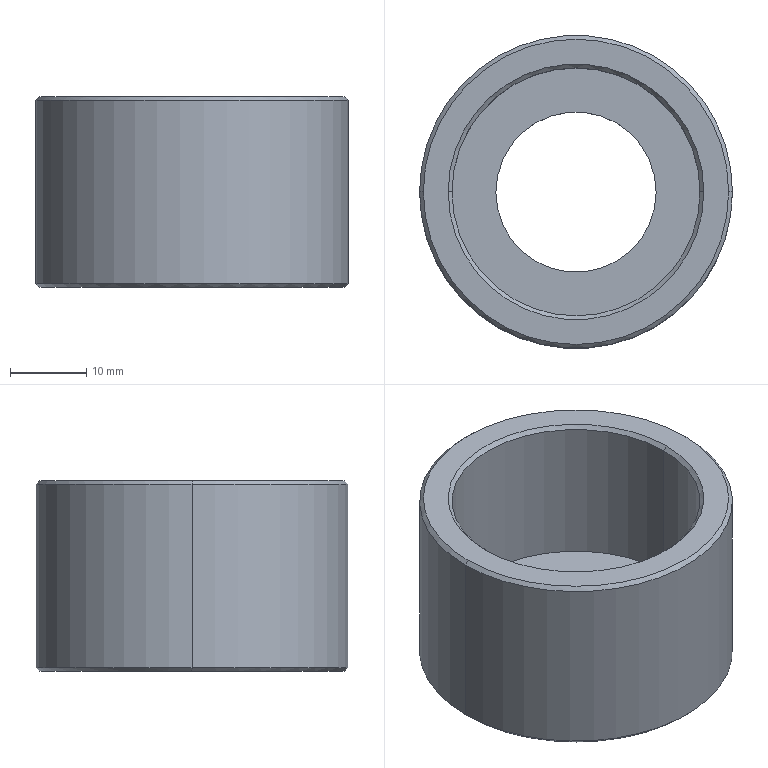Part | SolidWorks | features Chamfer 2, ICE 2, Extrusion 1 | 1 solid | 15 faces | box 41 x 41 x 25 mm | volume 14638 mm3 | cylinder 6 | cone 6 | plane 3 | commonest cylinder face diameters 21 x2 32.5 x2 41 x2
STEP:
#1=CARTESIAN_POINT('',(-10.5,0.,5.));
#2=VERTEX_POINT('',#1);
#3=CARTESIAN_POINT('',(10.5,0.,5.));
#4=VERTEX_POINT('',#3);
#5=CARTESIAN_POINT('',(0.,0.,5.));
#6=DIRECTION('',(0.,0.,1.));
#7=DIRECTION('',(1.,0.,0.));
#8=AXIS2_PLACEMENT_3D('',#5,#6,#7);
#9=CIRCLE('',#8,10.5);
#10=EDGE_CURVE('',#2,#4,#9,.T.);
#11=ORIENTED_EDGE('',*,*,#10,.T.);
#12=CARTESIAN_POINT('',(10.5,0.,0.));
#13=VERTEX_POINT('',#12);
#14=CARTESIAN_POINT('',(10.5,0.,31.));
#15=DIRECTION('',(0.,0.,-1.));
#16=VECTOR('',#15,1000.);
#17=LINE('',#14,#16);
#18=EDGE_CURVE('',#4,#13,#17,.T.);
#19=ORIENTED_EDGE('',*,*,#18,.T.);
#20=CARTESIAN_POINT('',(-10.5,0.,0.));
#21=VERTEX_POINT('',#20);
#22=CARTESIAN_POINT('',(0.,0.,0.));
#23=DIRECTION('',(0.,0.,-1.));
#24=DIRECTION('',(-1.,0.,0.));
#25=AXIS2_PLACEMENT_3D('',#22,#23,#24);
#26=CIRCLE('',#25,10.5);
#27=EDGE_CURVE('',#13,#21,#26,.T.);
#28=ORIENTED_EDGE('',*,*,#27,.T.);
#29=CARTESIAN_POINT('',(-10.5,0.,31.));
#30=DIRECTION('',(0.,0.,-1.));
#31=VECTOR('',#30,1000.);
#32=LINE('',#29,#31);
#33=EDGE_CURVE('',#2,#21,#32,.T.);
#34=ORIENTED_EDGE('',*,*,#33,.F.);
#35=EDGE_LOOP('',(#11,#19,#28,#34));
#36=FACE_OUTER_BOUND('',#35,.T.);
#37=CARTESIAN_POINT('',(0.,0.,31.));
#38=DIRECTION('',(0.,0.,-1.));
#39=DIRECTION('',(-1.,0.,0.));
#40=AXIS2_PLACEMENT_3D('',#37,#38,#39);
#41=CYLINDRICAL_SURFACE('',#40,10.5);
#42=ADVANCED_FACE('',(#36),#41,.F.);
#43=CARTESIAN_POINT('',(-16.25,0.,24.5));
#44=VERTEX_POINT('',#43);
#45=CARTESIAN_POINT('',(16.25,0.,24.5));
#46=VERTEX_POINT('',#45);
#47=CARTESIAN_POINT('',(0.,0.,24.5));
#48=DIRECTION('',(0.,0.,1.));
#49=DIRECTION('',(1.,0.,0.));
#50=AXIS2_PLACEMENT_3D('',#47,#48,#49);
#51=CIRCLE('',#50,16.25);
#52=EDGE_CURVE('',#44,#46,#51,.T.);
#53=ORIENTED_EDGE('',*,*,#52,.F.);
#54=CARTESIAN_POINT('',(-16.75,0.,25.));
#55=VERTEX_POINT('',#54);
#56=CARTESIAN_POINT('',(-16.25,0.,24.5));
#57=DIRECTION('',(-0.7071,0.,0.7071));
#58=VECTOR('',#57,1000.);
#59=LINE('',#56,#58);
#60=EDGE_CURVE('',#44,#55,#59,.T.);
#61=ORIENTED_EDGE('',*,*,#60,.T.);
#62=CARTESIAN_POINT('',(16.75,0.,25.));
#63=VERTEX_POINT('',#62);
#64=CARTESIAN_POINT('',(0.,0.,25.));
#65=DIRECTION('',(0.,0.,-1.));
#66=DIRECTION('',(1.,0.,0.));
#67=AXIS2_PLACEMENT_3D('',#64,#65,#66);
#68=CIRCLE('',#67,16.75);
#69=EDGE_CURVE('',#63,#55,#68,.T.);
#70=ORIENTED_EDGE('',*,*,#69,.F.);
#71=CARTESIAN_POINT('',(16.25,0.,24.5));
#72=DIRECTION('',(0.7071,0.,0.7071));
#73=VECTOR('',#72,1000.);
#74=LINE('',#71,#73);
#75=EDGE_CURVE('',#46,#63,#74,.T.);
#76=ORIENTED_EDGE('',*,*,#75,.F.);
#77=EDGE_LOOP('',(#53,#61,#70,#76));
#78=FACE_OUTER_BOUND('',#77,.T.);
#79=CARTESIAN_POINT('',(0.,0.,24.5));
#80=DIRECTION('',(0.,0.,1.));
#81=DIRECTION('',(1.,0.,0.));
#82=AXIS2_PLACEMENT_3D('',#79,#80,#81);
#83=CONICAL_SURFACE('',#82,16.25,0.7854);
#84=ADVANCED_FACE('',(#78),#83,.F.);
#85=CARTESIAN_POINT('',(-16.25,0.,5.));
#86=VERTEX_POINT('',#85);
#87=CARTESIAN_POINT('',(16.25,0.,5.));
#88=VERTEX_POINT('',#87);
#89=CARTESIAN_POINT('',(0.,0.,5.));
#90=DIRECTION('',(0.,0.,1.));
#91=DIRECTION('',(1.,0.,0.));
#92=AXIS2_PLACEMENT_3D('',#89,#90,#91);
#93=CIRCLE('',#92,16.25);
#94=EDGE_CURVE('',#86,#88,#93,.T.);
#95=ORIENTED_EDGE('',*,*,#94,.F.);
#96=CARTESIAN_POINT('',(-16.25,0.,5.));
#97=DIRECTION('',(0.,0.,1.));
#98=VECTOR('',#97,1000.);
#99=LINE('',#96,#98);
#100=EDGE_CURVE('',#86,#44,#99,.T.);
#101=ORIENTED_EDGE('',*,*,#100,.T.);
#102=ORIENTED_EDGE('',*,*,#52,.T.);
#103=CARTESIAN_POINT('',(16.25,0.,5.));
#104=DIRECTION('',(0.,0.,1.));
#105=VECTOR('',#104,1000.);
#106=LINE('',#103,#105);
#107=EDGE_CURVE('',#88,#46,#106,.T.);
#108=ORIENTED_EDGE('',*,*,#107,.F.);
#109=EDGE_LOOP('',(#95,#101,#102,#108));
#110=FACE_OUTER_BOUND('',#109,.T.);
#111=CARTESIAN_POINT('',(0.,0.,5.));
#112=DIRECTION('',(0.,0.,1.));
#113=DIRECTION('',(1.,0.,0.));
#114=AXIS2_PLACEMENT_3D('',#111,#112,#113);
#115=CYLINDRICAL_SURFACE('',#114,16.25);
#116=ADVANCED_FACE('',(#110),#115,.F.);
#117=CARTESIAN_POINT('',(-20.,0.,0.));
#118=VERTEX_POINT('',#117);
#119=CARTESIAN_POINT('',(20.,0.,0.));
#120=VERTEX_POINT('',#119);
#121=CARTESIAN_POINT('',(0.,0.,0.));
#122=DIRECTION('',(0.,0.,-1.));
#123=DIRECTION('',(1.,0.,0.));
#124=AXIS2_PLACEMENT_3D('',#121,#122,#123);
#125=CIRCLE('',#124,20.);
#126=EDGE_CURVE('',#118,#120,#125,.T.);
#127=ORIENTED_EDGE('',*,*,#126,.F.);
#128=CARTESIAN_POINT('',(-20.5,0.,0.5));
#129=VERTEX_POINT('',#128);
#130=CARTESIAN_POINT('',(-20.5,0.,0.5));
#131=DIRECTION('',(-0.7071,0.,0.7071));
#132=VECTOR('',#131,1000.);
#133=LINE('',#130,#132);
#134=EDGE_CURVE('',#118,#129,#133,.T.);
#135=ORIENTED_EDGE('',*,*,#134,.T.);
#136=CARTESIAN_POINT('',(20.5,0.,0.5));
#137=VERTEX_POINT('',#136);
#138=CARTESIAN_POINT('',(0.,0.,0.5));
#139=DIRECTION('',(0.,0.,1.));
#140=DIRECTION('',(1.,0.,0.));
#141=AXIS2_PLACEMENT_3D('',#138,#139,#140);
#142=CIRCLE('',#141,20.5);
#143=EDGE_CURVE('',#137,#129,#142,.T.);
#144=ORIENTED_EDGE('',*,*,#143,.F.);
#145=CARTESIAN_POINT('',(20.5,0.,0.5));
#146=DIRECTION('',(0.7071,0.,0.7071));
#147=VECTOR('',#146,1000.);
#148=LINE('',#145,#147);
#149=EDGE_CURVE('',#120,#137,#148,.T.);
#150=ORIENTED_EDGE('',*,*,#149,.F.);
#151=EDGE_LOOP('',(#127,#135,#144,#150));
#152=FACE_OUTER_BOUND('',#151,.T.);
#153=CARTESIAN_POINT('',(0.,0.,0.5));
#154=DIRECTION('',(0.,0.,1.));
#155=DIRECTION('',(1.,0.,0.));
#156=AXIS2_PLACEMENT_3D('',#153,#154,#155);
#157=CONICAL_SURFACE('',#156,20.5,0.7854);
#158=ADVANCED_FACE('',(#152),#157,.T.);
#159=CARTESIAN_POINT('',(20.,0.,25.));
#160=VERTEX_POINT('',#159);
#161=CARTESIAN_POINT('',(-20.,0.,25.));
#162=VERTEX_POINT('',#161);
#163=CARTESIAN_POINT('',(0.,0.,25.));
#164=DIRECTION('',(0.,0.,1.));
#165=DIRECTION('',(1.,0.,0.));
#166=AXIS2_PLACEMENT_3D('',#163,#164,#165);
#167=CIRCLE('',#166,20.);
#168=EDGE_CURVE('',#160,#162,#167,.T.);
#169=ORIENTED_EDGE('',*,*,#168,.F.);
#170=CARTESIAN_POINT('',(20.5,0.,24.5));
#171=VERTEX_POINT('',#170);
#172=CARTESIAN_POINT('',(20.,0.,25.));
#173=DIRECTION('',(0.7071,0.,-0.7071));
#174=VECTOR('',#173,1000.);
#175=LINE('',#172,#174);
#176=EDGE_CURVE('',#160,#171,#175,.T.);
#177=ORIENTED_EDGE('',*,*,#176,.T.);
#178=CARTESIAN_POINT('',(-20.5,0.,24.5));
#179=VERTEX_POINT('',#178);
#180=CARTESIAN_POINT('',(0.,0.,24.5));
#181=DIRECTION('',(0.,0.,-1.));
#182=DIRECTION('',(1.,0.,0.));
#183=AXIS2_PLACEMENT_3D('',#180,#181,#182);
#184=CIRCLE('',#183,20.5);
#185=EDGE_CURVE('',#179,#171,#184,.T.);
#186=ORIENTED_EDGE('',*,*,#185,.F.);
#187=CARTESIAN_POINT('',(-20.,0.,25.));
#188=DIRECTION('',(-0.7071,0.,-0.7071));
#189=VECTOR('',#188,1000.);
#190=LINE('',#187,#189);
#191=EDGE_CURVE('',#162,#179,#190,.T.);
#192=ORIENTED_EDGE('',*,*,#191,.F.);
#193=EDGE_LOOP('',(#169,#177,#186,#192));
#194=FACE_OUTER_BOUND('',#193,.T.);
#195=CARTESIAN_POINT('',(0.,0.,25.));
#196=DIRECTION('',(0.,0.,-1.));
#197=DIRECTION('',(-1.,0.,0.));
#198=AXIS2_PLACEMENT_3D('',#195,#196,#197);
#199=CONICAL_SURFACE('',#198,20.,0.7854);
#200=ADVANCED_FACE('',(#194),#199,.T.);
#201=ORIENTED_EDGE('',*,*,#185,.T.);
#202=CARTESIAN_POINT('',(20.5,0.,25.));
#203=DIRECTION('',(0.,0.,-1.));
#204=VECTOR('',#203,1000.);
#205=LINE('',#202,#204);
#206=EDGE_CURVE('',#171,#137,#205,.T.);
#207=ORIENTED_EDGE('',*,*,#206,.T.);
#208=ORIENTED_EDGE('',*,*,#143,.T.);
#209=CARTESIAN_POINT('',(-20.5,0.,25.));
#210=DIRECTION('',(0.,0.,-1.));
#211=VECTOR('',#210,1000.);
#212=LINE('',#209,#211);
#213=EDGE_CURVE('',#179,#129,#212,.T.);
#214=ORIENTED_EDGE('',*,*,#213,.F.);
#215=EDGE_LOOP('',(#201,#207,#208,#214));
#216=FACE_OUTER_BOUND('',#215,.T.);
#217=CARTESIAN_POINT('',(0.,0.,25.));
#218=DIRECTION('',(0.,0.,-1.));
#219=DIRECTION('',(-1.,0.,0.));
#220=AXIS2_PLACEMENT_3D('',#217,#218,#219);
#221=CYLINDRICAL_SURFACE('',#220,20.5);
#222=ADVANCED_FACE('',(#216),#221,.T.);
#223=ORIENTED_EDGE('',*,*,#206,.F.);
#224=CARTESIAN_POINT('',(0.,0.,24.5));
#225=DIRECTION('',(0.,0.,-1.));
#226=DIRECTION('',(1.,0.,0.));
#227=AXIS2_PLACEMENT_3D('',#224,#225,#226);
#228=CIRCLE('',#227,20.5);
#229=EDGE_CURVE('',#171,#179,#228,.T.);
#230=ORIENTED_EDGE('',*,*,#229,.T.);
#231=ORIENTED_EDGE('',*,*,#213,.T.);
#232=CARTESIAN_POINT('',(0.,0.,0.5));
#233=DIRECTION('',(0.,0.,1.));
#234=DIRECTION('',(1.,0.,0.));
#235=AXIS2_PLACEMENT_3D('',#232,#233,#234);
#236=CIRCLE('',#235,20.5);
#237=EDGE_CURVE('',#129,#137,#236,.T.);
#238=ORIENTED_EDGE('',*,*,#237,.T.);
#239=EDGE_LOOP('',(#223,#230,#231,#238));
#240=FACE_OUTER_BOUND('',#239,.T.);
#241=CARTESIAN_POINT('',(0.,0.,25.));
#242=DIRECTION('',(0.,0.,-1.));
#243=DIRECTION('',(-1.,0.,0.));
#244=AXIS2_PLACEMENT_3D('',#241,#242,#243);
#245=CYLINDRICAL_SURFACE('',#244,20.5);
#246=ADVANCED_FACE('',(#240),#245,.T.);
#247=ORIENTED_EDGE('',*,*,#69,.T.);
#248=CARTESIAN_POINT('',(0.,0.,25.));
#249=DIRECTION('',(0.,0.,-1.));
#250=DIRECTION('',(1.,0.,0.));
#251=AXIS2_PLACEMENT_3D('',#248,#249,#250);
#252=CIRCLE('',#251,16.75);
#253=EDGE_CURVE('',#55,#63,#252,.T.);
#254=ORIENTED_EDGE('',*,*,#253,.T.);
#255=EDGE_LOOP('',(#247,#254));
#256=FACE_BOUND('',#255,.T.);
#257=CARTESIAN_POINT('',(0.,0.,25.));
#258=DIRECTION('',(0.,0.,1.));
#259=DIRECTION('',(1.,0.,0.));
#260=AXIS2_PLACEMENT_3D('',#257,#258,#259);
#261=CIRCLE('',#260,20.);
#262=EDGE_CURVE('',#162,#160,#261,.T.);
#263=ORIENTED_EDGE('',*,*,#262,.T.);
#264=ORIENTED_EDGE('',*,*,#168,.T.);
#265=EDGE_LOOP('',(#263,#264));
#266=FACE_OUTER_BOUND('',#265,.T.);
#267=CARTESIAN_POINT('',(0.,0.,25.));
#268=DIRECTION('',(0.,0.,1.));
#269=DIRECTION('',(1.,0.,0.));
#270=AXIS2_PLACEMENT_3D('',#267,#268,#269);
#271=PLANE('',#270);
#272=ADVANCED_FACE('',(#256,#266),#271,.T.);
#273=CARTESIAN_POINT('',(0.,0.,0.));
#274=DIRECTION('',(0.,0.,-1.));
#275=DIRECTION('',(-1.,0.,0.));
#276=AXIS2_PLACEMENT_3D('',#273,#274,#275);
#277=CIRCLE('',#276,10.5);
#278=EDGE_CURVE('',#21,#13,#277,.T.);
#279=ORIENTED_EDGE('',*,*,#278,.F.);
#280=ORIENTED_EDGE('',*,*,#27,.F.);
#281=EDGE_LOOP('',(#279,#280));
#282=FACE_BOUND('',#281,.T.);
#283=CARTESIAN_POINT('',(0.,0.,0.));
#284=DIRECTION('',(0.,0.,-1.));
#285=DIRECTION('',(1.,0.,0.));
#286=AXIS2_PLACEMENT_3D('',#283,#284,#285);
#287=CIRCLE('',#286,20.);
#288=EDGE_CURVE('',#120,#118,#287,.T.);
#289=ORIENTED_EDGE('',*,*,#288,.T.);
#290=ORIENTED_EDGE('',*,*,#126,.T.);
#291=EDGE_LOOP('',(#289,#290));
#292=FACE_OUTER_BOUND('',#291,.T.);
#293=CARTESIAN_POINT('',(0.,0.,0.));
#294=DIRECTION('',(0.,0.,1.));
#295=DIRECTION('',(1.,0.,0.));
#296=AXIS2_PLACEMENT_3D('',#293,#294,#295);
#297=PLANE('',#296);
#298=ADVANCED_FACE('',(#282,#292),#297,.F.);
#299=ORIENTED_EDGE('',*,*,#176,.F.);
#300=ORIENTED_EDGE('',*,*,#262,.F.);
#301=ORIENTED_EDGE('',*,*,#191,.T.);
#302=ORIENTED_EDGE('',*,*,#229,.F.);
#303=EDGE_LOOP('',(#299,#300,#301,#302));
#304=FACE_OUTER_BOUND('',#303,.T.);
#305=CARTESIAN_POINT('',(0.,0.,25.));
#306=DIRECTION('',(0.,0.,-1.));
#307=DIRECTION('',(-1.,0.,0.));
#308=AXIS2_PLACEMENT_3D('',#305,#306,#307);
#309=CONICAL_SURFACE('',#308,20.,0.7854);
#310=ADVANCED_FACE('',(#304),#309,.T.);
#311=ORIENTED_EDGE('',*,*,#134,.F.);
#312=ORIENTED_EDGE('',*,*,#288,.F.);
#313=ORIENTED_EDGE('',*,*,#149,.T.);
#314=ORIENTED_EDGE('',*,*,#237,.F.);
#315=EDGE_LOOP('',(#311,#312,#313,#314));
#316=FACE_OUTER_BOUND('',#315,.T.);
#317=CARTESIAN_POINT('',(0.,0.,0.5));
#318=DIRECTION('',(0.,0.,1.));
#319=DIRECTION('',(1.,0.,0.));
#320=AXIS2_PLACEMENT_3D('',#317,#318,#319);
#321=CONICAL_SURFACE('',#320,20.5,0.7854);
#322=ADVANCED_FACE('',(#316),#321,.T.);
#323=ORIENTED_EDGE('',*,*,#100,.F.);
#324=CARTESIAN_POINT('',(0.,0.,5.));
#325=DIRECTION('',(0.,0.,1.));
#326=DIRECTION('',(1.,0.,0.));
#327=AXIS2_PLACEMENT_3D('',#324,#325,#326);
#328=CIRCLE('',#327,16.25);
#329=EDGE_CURVE('',#88,#86,#328,.T.);
#330=ORIENTED_EDGE('',*,*,#329,.F.);
#331=ORIENTED_EDGE('',*,*,#107,.T.);
#332=CARTESIAN_POINT('',(0.,0.,24.5));
#333=DIRECTION('',(0.,0.,1.));
#334=DIRECTION('',(1.,0.,0.));
#335=AXIS2_PLACEMENT_3D('',#332,#333,#334);
#336=CIRCLE('',#335,16.25);
#337=EDGE_CURVE('',#46,#44,#336,.T.);
#338=ORIENTED_EDGE('',*,*,#337,.T.);
#339=EDGE_LOOP('',(#323,#330,#331,#338));
#340=FACE_OUTER_BOUND('',#339,.T.);
#341=CARTESIAN_POINT('',(0.,0.,5.));
#342=DIRECTION('',(0.,0.,1.));
#343=DIRECTION('',(1.,0.,0.));
#344=AXIS2_PLACEMENT_3D('',#341,#342,#343);
#345=CYLINDRICAL_SURFACE('',#344,16.25);
#346=ADVANCED_FACE('',(#340),#345,.F.);
#347=ORIENTED_EDGE('',*,*,#10,.F.);
#348=CARTESIAN_POINT('',(0.,0.,5.));
#349=DIRECTION('',(0.,0.,1.));
#350=DIRECTION('',(1.,0.,0.));
#351=AXIS2_PLACEMENT_3D('',#348,#349,#350);
#352=CIRCLE('',#351,10.5);
#353=EDGE_CURVE('',#4,#2,#352,.T.);
#354=ORIENTED_EDGE('',*,*,#353,.F.);
#355=EDGE_LOOP('',(#347,#354));
#356=FACE_BOUND('',#355,.T.);
#357=ORIENTED_EDGE('',*,*,#329,.T.);
#358=ORIENTED_EDGE('',*,*,#94,.T.);
#359=EDGE_LOOP('',(#357,#358));
#360=FACE_OUTER_BOUND('',#359,.T.);
#361=CARTESIAN_POINT('',(0.,0.,5.));
#362=DIRECTION('',(0.,0.,1.));
#363=DIRECTION('',(1.,0.,0.));
#364=AXIS2_PLACEMENT_3D('',#361,#362,#363);
#365=PLANE('',#364);
#366=ADVANCED_FACE('',(#356,#360),#365,.T.);
#367=ORIENTED_EDGE('',*,*,#60,.F.);
#368=ORIENTED_EDGE('',*,*,#337,.F.);
#369=ORIENTED_EDGE('',*,*,#75,.T.);
#370=ORIENTED_EDGE('',*,*,#253,.F.);
#371=EDGE_LOOP('',(#367,#368,#369,#370));
#372=FACE_OUTER_BOUND('',#371,.T.);
#373=CARTESIAN_POINT('',(0.,0.,24.5));
#374=DIRECTION('',(0.,0.,1.));
#375=DIRECTION('',(1.,0.,0.));
#376=AXIS2_PLACEMENT_3D('',#373,#374,#375);
#377=CONICAL_SURFACE('',#376,16.25,0.7854);
#378=ADVANCED_FACE('',(#372),#377,.F.);
#379=ORIENTED_EDGE('',*,*,#18,.F.);
#380=ORIENTED_EDGE('',*,*,#353,.T.);
#381=ORIENTED_EDGE('',*,*,#33,.T.);
#382=ORIENTED_EDGE('',*,*,#278,.T.);
#383=EDGE_LOOP('',(#379,#380,#381,#382));
#384=FACE_OUTER_BOUND('',#383,.T.);
#385=CARTESIAN_POINT('',(0.,0.,31.));
#386=DIRECTION('',(0.,0.,-1.));
#387=DIRECTION('',(-1.,0.,0.));
#388=AXIS2_PLACEMENT_3D('',#385,#386,#387);
#389=CYLINDRICAL_SURFACE('',#388,10.5);
#390=ADVANCED_FACE('',(#384),#389,.F.);
#391=CLOSED_SHELL('',(#42,#84,#116,#158,#200,#222,#246,#272,#298,#310,#322,#346,#366,#378,#390));
#392=MANIFOLD_SOLID_BREP('',#391);
#393=CARTESIAN_POINT('',(0.,0.,0.));
#394=DIRECTION('',(0.,0.,1.));
#395=DIRECTION('',(1.,0.,0.));
#396=AXIS2_PLACEMENT_3D('',#393,#394,#395);
#397=(LENGTH_UNIT()NAMED_UNIT(*)SI_UNIT(.MILLI.,.METRE.));
#398=UNCERTAINTY_MEASURE_WITH_UNIT(LENGTH_MEASURE(0.00001),#397,'','');
#399=(NAMED_UNIT(*)PLANE_ANGLE_UNIT()SI_UNIT($,.RADIAN.));
#400=(NAMED_UNIT(*)SI_UNIT($,.STERADIAN.)SOLID_ANGLE_UNIT());
#401=(GEOMETRIC_REPRESENTATION_CONTEXT(3)GLOBAL_UNCERTAINTY_ASSIGNED_CONTEXT((#398))GLOBAL_UNIT_ASSIGNED_CONTEXT((#397,#399,#400))REPRESENTATION_CONTEXT('',''));
#402=ADVANCED_BREP_SHAPE_REPRESENTATION('',(#392,#396),#401);